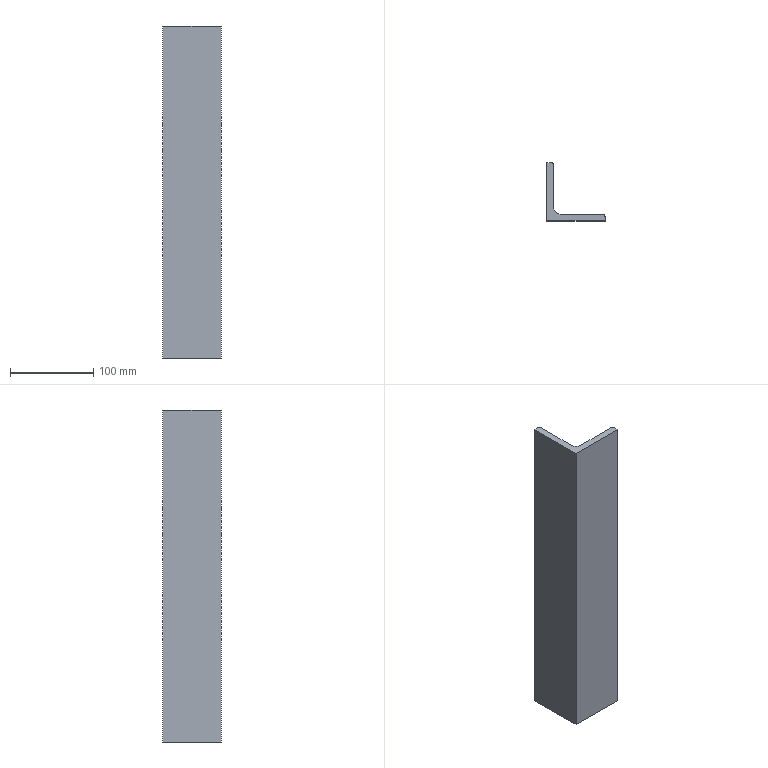Part | SolidWorks | features Extrusion 1 | 1 solid | 11 faces | box 70 x 70 x 400 mm | volume 426349 mm3 | plane 8 | cylinder 3 | commonest cylinder face diameters 6 x2 16 x1
STEP:
#1=CARTESIAN_POINT('',(5.,70.,0.));
#2=VERTEX_POINT('',#1);
#3=CARTESIAN_POINT('',(0.,70.,0.));
#4=VERTEX_POINT('',#3);
#5=CARTESIAN_POINT('',(5.,70.,0.));
#6=DIRECTION('',(-1.,0.,0.));
#7=VECTOR('',#6,1000.);
#8=LINE('',#5,#7);
#9=EDGE_CURVE('',#2,#4,#8,.T.);
#10=ORIENTED_EDGE('',*,*,#9,.T.);
#11=CARTESIAN_POINT('',(0.,70.,400.));
#12=VERTEX_POINT('',#11);
#13=CARTESIAN_POINT('',(0.,70.,400.));
#14=DIRECTION('',(0.,0.,-1.));
#15=VECTOR('',#14,1000.);
#16=LINE('',#13,#15);
#17=EDGE_CURVE('',#12,#4,#16,.T.);
#18=ORIENTED_EDGE('',*,*,#17,.F.);
#19=CARTESIAN_POINT('',(5.,70.,400.));
#20=VERTEX_POINT('',#19);
#21=CARTESIAN_POINT('',(5.,70.,400.));
#22=DIRECTION('',(-1.,0.,0.));
#23=VECTOR('',#22,1000.);
#24=LINE('',#21,#23);
#25=EDGE_CURVE('',#20,#12,#24,.T.);
#26=ORIENTED_EDGE('',*,*,#25,.F.);
#27=CARTESIAN_POINT('',(5.,70.,400.));
#28=DIRECTION('',(0.,0.,-1.));
#29=VECTOR('',#28,1000.);
#30=LINE('',#27,#29);
#31=EDGE_CURVE('',#20,#2,#30,.T.);
#32=ORIENTED_EDGE('',*,*,#31,.T.);
#33=EDGE_LOOP('',(#10,#18,#26,#32));
#34=FACE_OUTER_BOUND('',#33,.T.);
#35=CARTESIAN_POINT('',(5.,70.,400.));
#36=DIRECTION('',(0.,-1.,0.));
#37=DIRECTION('',(0.,0.,-1.));
#38=AXIS2_PLACEMENT_3D('',#35,#36,#37);
#39=PLANE('',#38);
#40=ADVANCED_FACE('',(#34),#39,.F.);
#41=CARTESIAN_POINT('',(0.,0.,0.));
#42=VERTEX_POINT('',#41);
#43=CARTESIAN_POINT('',(0.,70.,0.));
#44=DIRECTION('',(0.,-1.,0.));
#45=VECTOR('',#44,1000.);
#46=LINE('',#43,#45);
#47=EDGE_CURVE('',#4,#42,#46,.T.);
#48=ORIENTED_EDGE('',*,*,#47,.T.);
#49=CARTESIAN_POINT('',(0.,0.,400.));
#50=VERTEX_POINT('',#49);
#51=CARTESIAN_POINT('',(0.,0.,400.));
#52=DIRECTION('',(0.,0.,-1.));
#53=VECTOR('',#52,1000.);
#54=LINE('',#51,#53);
#55=EDGE_CURVE('',#50,#42,#54,.T.);
#56=ORIENTED_EDGE('',*,*,#55,.F.);
#57=CARTESIAN_POINT('',(0.,70.,400.));
#58=DIRECTION('',(0.,-1.,0.));
#59=VECTOR('',#58,1000.);
#60=LINE('',#57,#59);
#61=EDGE_CURVE('',#12,#50,#60,.T.);
#62=ORIENTED_EDGE('',*,*,#61,.F.);
#63=ORIENTED_EDGE('',*,*,#17,.T.);
#64=EDGE_LOOP('',(#48,#56,#62,#63));
#65=FACE_OUTER_BOUND('',#64,.T.);
#66=CARTESIAN_POINT('',(0.,70.,400.));
#67=DIRECTION('',(1.,0.,0.));
#68=DIRECTION('',(0.,0.,-1.));
#69=AXIS2_PLACEMENT_3D('',#66,#67,#68);
#70=PLANE('',#69);
#71=ADVANCED_FACE('',(#65),#70,.F.);
#72=CARTESIAN_POINT('',(70.,0.,0.));
#73=VERTEX_POINT('',#72);
#74=CARTESIAN_POINT('',(0.,0.,0.));
#75=DIRECTION('',(1.,0.,0.));
#76=VECTOR('',#75,1000.);
#77=LINE('',#74,#76);
#78=EDGE_CURVE('',#42,#73,#77,.T.);
#79=ORIENTED_EDGE('',*,*,#78,.T.);
#80=CARTESIAN_POINT('',(70.,0.,400.));
#81=VERTEX_POINT('',#80);
#82=CARTESIAN_POINT('',(70.,0.,400.));
#83=DIRECTION('',(0.,0.,-1.));
#84=VECTOR('',#83,1000.);
#85=LINE('',#82,#84);
#86=EDGE_CURVE('',#81,#73,#85,.T.);
#87=ORIENTED_EDGE('',*,*,#86,.F.);
#88=CARTESIAN_POINT('',(0.,0.,400.));
#89=DIRECTION('',(1.,0.,0.));
#90=VECTOR('',#89,1000.);
#91=LINE('',#88,#90);
#92=EDGE_CURVE('',#50,#81,#91,.T.);
#93=ORIENTED_EDGE('',*,*,#92,.F.);
#94=ORIENTED_EDGE('',*,*,#55,.T.);
#95=EDGE_LOOP('',(#79,#87,#93,#94));
#96=FACE_OUTER_BOUND('',#95,.T.);
#97=CARTESIAN_POINT('',(0.,0.,400.));
#98=DIRECTION('',(0.,1.,0.));
#99=DIRECTION('',(0.,0.,1.));
#100=AXIS2_PLACEMENT_3D('',#97,#98,#99);
#101=PLANE('',#100);
#102=ADVANCED_FACE('',(#96),#101,.F.);
#103=CARTESIAN_POINT('',(70.,5.,0.));
#104=VERTEX_POINT('',#103);
#105=CARTESIAN_POINT('',(70.,0.,0.));
#106=DIRECTION('',(0.,1.,0.));
#107=VECTOR('',#106,1000.);
#108=LINE('',#105,#107);
#109=EDGE_CURVE('',#73,#104,#108,.T.);
#110=ORIENTED_EDGE('',*,*,#109,.T.);
#111=CARTESIAN_POINT('',(70.,5.,400.));
#112=VERTEX_POINT('',#111);
#113=CARTESIAN_POINT('',(70.,5.,400.));
#114=DIRECTION('',(0.,0.,-1.));
#115=VECTOR('',#114,1000.);
#116=LINE('',#113,#115);
#117=EDGE_CURVE('',#112,#104,#116,.T.);
#118=ORIENTED_EDGE('',*,*,#117,.F.);
#119=CARTESIAN_POINT('',(70.,0.,400.));
#120=DIRECTION('',(0.,1.,0.));
#121=VECTOR('',#120,1000.);
#122=LINE('',#119,#121);
#123=EDGE_CURVE('',#81,#112,#122,.T.);
#124=ORIENTED_EDGE('',*,*,#123,.F.);
#125=ORIENTED_EDGE('',*,*,#86,.T.);
#126=EDGE_LOOP('',(#110,#118,#124,#125));
#127=FACE_OUTER_BOUND('',#126,.T.);
#128=CARTESIAN_POINT('',(70.,0.,400.));
#129=DIRECTION('',(-1.,0.,0.));
#130=DIRECTION('',(0.,0.,1.));
#131=AXIS2_PLACEMENT_3D('',#128,#129,#130);
#132=PLANE('',#131);
#133=ADVANCED_FACE('',(#127),#132,.F.);
#134=CARTESIAN_POINT('',(67.,8.,0.));
#135=VERTEX_POINT('',#134);
#136=CARTESIAN_POINT('',(67.,5.,0.));
#137=DIRECTION('',(0.,0.,1.));
#138=DIRECTION('',(1.,0.,0.));
#139=AXIS2_PLACEMENT_3D('',#136,#137,#138);
#140=CIRCLE('',#139,3.);
#141=EDGE_CURVE('',#104,#135,#140,.T.);
#142=ORIENTED_EDGE('',*,*,#141,.T.);
#143=CARTESIAN_POINT('',(67.,8.,400.));
#144=VERTEX_POINT('',#143);
#145=CARTESIAN_POINT('',(67.,8.,400.));
#146=DIRECTION('',(0.,0.,-1.));
#147=VECTOR('',#146,1000.);
#148=LINE('',#145,#147);
#149=EDGE_CURVE('',#144,#135,#148,.T.);
#150=ORIENTED_EDGE('',*,*,#149,.F.);
#151=CARTESIAN_POINT('',(67.,5.,400.));
#152=DIRECTION('',(0.,0.,1.));
#153=DIRECTION('',(1.,0.,0.));
#154=AXIS2_PLACEMENT_3D('',#151,#152,#153);
#155=CIRCLE('',#154,3.);
#156=EDGE_CURVE('',#112,#144,#155,.T.);
#157=ORIENTED_EDGE('',*,*,#156,.F.);
#158=ORIENTED_EDGE('',*,*,#117,.T.);
#159=EDGE_LOOP('',(#142,#150,#157,#158));
#160=FACE_OUTER_BOUND('',#159,.T.);
#161=CARTESIAN_POINT('',(67.,5.,400.));
#162=DIRECTION('',(0.,0.,-1.));
#163=DIRECTION('',(-1.,0.,0.));
#164=AXIS2_PLACEMENT_3D('',#161,#162,#163);
#165=CYLINDRICAL_SURFACE('',#164,3.);
#166=ADVANCED_FACE('',(#160),#165,.T.);
#167=CARTESIAN_POINT('',(16.,8.,0.));
#168=VERTEX_POINT('',#167);
#169=CARTESIAN_POINT('',(67.,8.,0.));
#170=DIRECTION('',(-1.,0.,0.));
#171=VECTOR('',#170,1000.);
#172=LINE('',#169,#171);
#173=EDGE_CURVE('',#135,#168,#172,.T.);
#174=ORIENTED_EDGE('',*,*,#173,.T.);
#175=CARTESIAN_POINT('',(16.,8.,400.));
#176=VERTEX_POINT('',#175);
#177=CARTESIAN_POINT('',(16.,8.,400.));
#178=DIRECTION('',(0.,0.,-1.));
#179=VECTOR('',#178,1000.);
#180=LINE('',#177,#179);
#181=EDGE_CURVE('',#176,#168,#180,.T.);
#182=ORIENTED_EDGE('',*,*,#181,.F.);
#183=CARTESIAN_POINT('',(67.,8.,400.));
#184=DIRECTION('',(-1.,0.,0.));
#185=VECTOR('',#184,1000.);
#186=LINE('',#183,#185);
#187=EDGE_CURVE('',#144,#176,#186,.T.);
#188=ORIENTED_EDGE('',*,*,#187,.F.);
#189=ORIENTED_EDGE('',*,*,#149,.T.);
#190=EDGE_LOOP('',(#174,#182,#188,#189));
#191=FACE_OUTER_BOUND('',#190,.T.);
#192=CARTESIAN_POINT('',(67.,8.,400.));
#193=DIRECTION('',(0.,-1.,0.));
#194=DIRECTION('',(1.,0.,0.));
#195=AXIS2_PLACEMENT_3D('',#192,#193,#194);
#196=PLANE('',#195);
#197=ADVANCED_FACE('',(#191),#196,.F.);
#198=CARTESIAN_POINT('',(8.,16.,0.));
#199=VERTEX_POINT('',#198);
#200=CARTESIAN_POINT('',(16.,16.,0.));
#201=DIRECTION('',(0.,0.,-1.));
#202=DIRECTION('',(-1.,0.,0.));
#203=AXIS2_PLACEMENT_3D('',#200,#201,#202);
#204=CIRCLE('',#203,8.);
#205=EDGE_CURVE('',#168,#199,#204,.T.);
#206=ORIENTED_EDGE('',*,*,#205,.T.);
#207=CARTESIAN_POINT('',(8.,16.,400.));
#208=VERTEX_POINT('',#207);
#209=CARTESIAN_POINT('',(8.,16.,400.));
#210=DIRECTION('',(0.,0.,-1.));
#211=VECTOR('',#210,1000.);
#212=LINE('',#209,#211);
#213=EDGE_CURVE('',#208,#199,#212,.T.);
#214=ORIENTED_EDGE('',*,*,#213,.F.);
#215=CARTESIAN_POINT('',(16.,16.,400.));
#216=DIRECTION('',(0.,0.,-1.));
#217=DIRECTION('',(-1.,0.,0.));
#218=AXIS2_PLACEMENT_3D('',#215,#216,#217);
#219=CIRCLE('',#218,8.);
#220=EDGE_CURVE('',#176,#208,#219,.T.);
#221=ORIENTED_EDGE('',*,*,#220,.F.);
#222=ORIENTED_EDGE('',*,*,#181,.T.);
#223=EDGE_LOOP('',(#206,#214,#221,#222));
#224=FACE_OUTER_BOUND('',#223,.T.);
#225=CARTESIAN_POINT('',(16.,16.,400.));
#226=DIRECTION('',(0.,0.,-1.));
#227=DIRECTION('',(-1.,0.,0.));
#228=AXIS2_PLACEMENT_3D('',#225,#226,#227);
#229=CYLINDRICAL_SURFACE('',#228,8.);
#230=ADVANCED_FACE('',(#224),#229,.F.);
#231=CARTESIAN_POINT('',(8.,67.,0.));
#232=VERTEX_POINT('',#231);
#233=CARTESIAN_POINT('',(8.,16.,0.));
#234=DIRECTION('',(0.,1.,0.));
#235=VECTOR('',#234,1000.);
#236=LINE('',#233,#235);
#237=EDGE_CURVE('',#199,#232,#236,.T.);
#238=ORIENTED_EDGE('',*,*,#237,.T.);
#239=CARTESIAN_POINT('',(8.,67.,400.));
#240=VERTEX_POINT('',#239);
#241=CARTESIAN_POINT('',(8.,67.,400.));
#242=DIRECTION('',(0.,0.,-1.));
#243=VECTOR('',#242,1000.);
#244=LINE('',#241,#243);
#245=EDGE_CURVE('',#240,#232,#244,.T.);
#246=ORIENTED_EDGE('',*,*,#245,.F.);
#247=CARTESIAN_POINT('',(8.,16.,400.));
#248=DIRECTION('',(0.,1.,0.));
#249=VECTOR('',#248,1000.);
#250=LINE('',#247,#249);
#251=EDGE_CURVE('',#208,#240,#250,.T.);
#252=ORIENTED_EDGE('',*,*,#251,.F.);
#253=ORIENTED_EDGE('',*,*,#213,.T.);
#254=EDGE_LOOP('',(#238,#246,#252,#253));
#255=FACE_OUTER_BOUND('',#254,.T.);
#256=CARTESIAN_POINT('',(8.,16.,400.));
#257=DIRECTION('',(-1.,0.,0.));
#258=DIRECTION('',(0.,-1.,0.));
#259=AXIS2_PLACEMENT_3D('',#256,#257,#258);
#260=PLANE('',#259);
#261=ADVANCED_FACE('',(#255),#260,.F.);
#262=CARTESIAN_POINT('',(5.,67.,0.));
#263=DIRECTION('',(0.,0.,1.));
#264=DIRECTION('',(1.,0.,0.));
#265=AXIS2_PLACEMENT_3D('',#262,#263,#264);
#266=CIRCLE('',#265,3.);
#267=EDGE_CURVE('',#232,#2,#266,.T.);
#268=ORIENTED_EDGE('',*,*,#267,.T.);
#269=ORIENTED_EDGE('',*,*,#31,.F.);
#270=CARTESIAN_POINT('',(5.,67.,400.));
#271=DIRECTION('',(0.,0.,1.));
#272=DIRECTION('',(1.,0.,0.));
#273=AXIS2_PLACEMENT_3D('',#270,#271,#272);
#274=CIRCLE('',#273,3.);
#275=EDGE_CURVE('',#240,#20,#274,.T.);
#276=ORIENTED_EDGE('',*,*,#275,.F.);
#277=ORIENTED_EDGE('',*,*,#245,.T.);
#278=EDGE_LOOP('',(#268,#269,#276,#277));
#279=FACE_OUTER_BOUND('',#278,.T.);
#280=CARTESIAN_POINT('',(5.,67.,400.));
#281=DIRECTION('',(0.,0.,-1.));
#282=DIRECTION('',(-1.,0.,0.));
#283=AXIS2_PLACEMENT_3D('',#280,#281,#282);
#284=CYLINDRICAL_SURFACE('',#283,3.);
#285=ADVANCED_FACE('',(#279),#284,.T.);
#286=ORIENTED_EDGE('',*,*,#25,.T.);
#287=ORIENTED_EDGE('',*,*,#61,.T.);
#288=ORIENTED_EDGE('',*,*,#92,.T.);
#289=ORIENTED_EDGE('',*,*,#123,.T.);
#290=ORIENTED_EDGE('',*,*,#156,.T.);
#291=ORIENTED_EDGE('',*,*,#187,.T.);
#292=ORIENTED_EDGE('',*,*,#220,.T.);
#293=ORIENTED_EDGE('',*,*,#251,.T.);
#294=ORIENTED_EDGE('',*,*,#275,.T.);
#295=EDGE_LOOP('',(#286,#287,#288,#289,#290,#291,#292,#293,#294));
#296=FACE_OUTER_BOUND('',#295,.T.);
#297=CARTESIAN_POINT('',(67.,5.,400.));
#298=DIRECTION('',(0.,0.,1.));
#299=DIRECTION('',(1.,0.,0.));
#300=AXIS2_PLACEMENT_3D('',#297,#298,#299);
#301=PLANE('',#300);
#302=ADVANCED_FACE('',(#296),#301,.T.);
#303=ORIENTED_EDGE('',*,*,#9,.F.);
#304=ORIENTED_EDGE('',*,*,#267,.F.);
#305=ORIENTED_EDGE('',*,*,#237,.F.);
#306=ORIENTED_EDGE('',*,*,#205,.F.);
#307=ORIENTED_EDGE('',*,*,#173,.F.);
#308=ORIENTED_EDGE('',*,*,#141,.F.);
#309=ORIENTED_EDGE('',*,*,#109,.F.);
#310=ORIENTED_EDGE('',*,*,#78,.F.);
#311=ORIENTED_EDGE('',*,*,#47,.F.);
#312=EDGE_LOOP('',(#303,#304,#305,#306,#307,#308,#309,#310,#311));
#313=FACE_OUTER_BOUND('',#312,.T.);
#314=CARTESIAN_POINT('',(67.,5.,0.));
#315=DIRECTION('',(0.,0.,1.));
#316=DIRECTION('',(1.,0.,0.));
#317=AXIS2_PLACEMENT_3D('',#314,#315,#316);
#318=PLANE('',#317);
#319=ADVANCED_FACE('',(#313),#318,.F.);
#320=CLOSED_SHELL('',(#40,#71,#102,#133,#166,#197,#230,#261,#285,#302,#319));
#321=MANIFOLD_SOLID_BREP('',#320);
#322=CARTESIAN_POINT('',(0.,0.,0.));
#323=DIRECTION('',(0.,0.,1.));
#324=DIRECTION('',(1.,0.,0.));
#325=AXIS2_PLACEMENT_3D('',#322,#323,#324);
#326=(LENGTH_UNIT()NAMED_UNIT(*)SI_UNIT(.MILLI.,.METRE.));
#327=UNCERTAINTY_MEASURE_WITH_UNIT(LENGTH_MEASURE(0.00001),#326,'','');
#328=(NAMED_UNIT(*)PLANE_ANGLE_UNIT()SI_UNIT($,.RADIAN.));
#329=(NAMED_UNIT(*)SI_UNIT($,.STERADIAN.)SOLID_ANGLE_UNIT());
#330=(GEOMETRIC_REPRESENTATION_CONTEXT(3)GLOBAL_UNCERTAINTY_ASSIGNED_CONTEXT((#327))GLOBAL_UNIT_ASSIGNED_CONTEXT((#326,#328,#329))REPRESENTATION_CONTEXT('',''));
#331=ADVANCED_BREP_SHAPE_REPRESENTATION('',(#321,#325),#330);